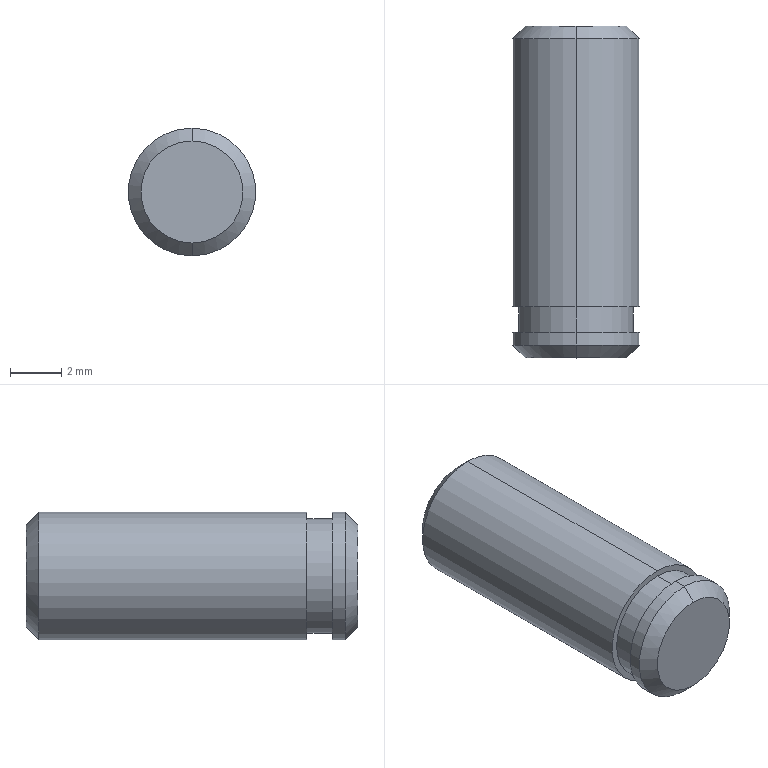Part | SolidWorks | features ICE 2, Chamfer 1, Extrusion 1 | 1 solid | 14 faces | box 5 x 13 x 5 mm | volume 247.859 mm3 | cylinder 6 | cone 4 | plane 4 | commonest cylinder face diameters 5 x4 4.5 x2
STEP:
#1=CARTESIAN_POINT('',(0.,13.,2.));
#2=VERTEX_POINT('',#1);
#3=CARTESIAN_POINT('',(0.,13.,-2.));
#4=VERTEX_POINT('',#3);
#5=CARTESIAN_POINT('',(0.,13.,0.));
#6=DIRECTION('',(0.,1.,0.));
#7=DIRECTION('',(0.,0.,1.));
#8=AXIS2_PLACEMENT_3D('',#5,#6,#7);
#9=CIRCLE('',#8,2.);
#10=EDGE_CURVE('',#2,#4,#9,.T.);
#11=ORIENTED_EDGE('',*,*,#10,.F.);
#12=CARTESIAN_POINT('',(0.,12.5,2.5));
#13=VERTEX_POINT('',#12);
#14=CARTESIAN_POINT('',(0.,13.,2.));
#15=DIRECTION('',(0.,-0.7071,0.7071));
#16=VECTOR('',#15,1000.);
#17=LINE('',#14,#16);
#18=EDGE_CURVE('',#2,#13,#17,.T.);
#19=ORIENTED_EDGE('',*,*,#18,.T.);
#20=CARTESIAN_POINT('',(0.,12.5,-2.5));
#21=VERTEX_POINT('',#20);
#22=CARTESIAN_POINT('',(0.,12.5,0.));
#23=DIRECTION('',(0.,-1.,0.));
#24=DIRECTION('',(0.,0.,1.));
#25=AXIS2_PLACEMENT_3D('',#22,#23,#24);
#26=CIRCLE('',#25,2.5);
#27=EDGE_CURVE('',#21,#13,#26,.T.);
#28=ORIENTED_EDGE('',*,*,#27,.F.);
#29=CARTESIAN_POINT('',(0.,13.,-2.));
#30=DIRECTION('',(0.,-0.7071,-0.7071));
#31=VECTOR('',#30,1000.);
#32=LINE('',#29,#31);
#33=EDGE_CURVE('',#4,#21,#32,.T.);
#34=ORIENTED_EDGE('',*,*,#33,.F.);
#35=EDGE_LOOP('',(#11,#19,#28,#34));
#36=FACE_OUTER_BOUND('',#35,.T.);
#37=CARTESIAN_POINT('',(0.,13.,0.));
#38=DIRECTION('',(0.,-1.,0.));
#39=DIRECTION('',(0.,0.,-1.));
#40=AXIS2_PLACEMENT_3D('',#37,#38,#39);
#41=CONICAL_SURFACE('',#40,2.,0.7854);
#42=ADVANCED_FACE('',(#36),#41,.T.);
#43=CARTESIAN_POINT('',(0.,0.,-2.));
#44=VERTEX_POINT('',#43);
#45=CARTESIAN_POINT('',(0.,0.,2.));
#46=VERTEX_POINT('',#45);
#47=CARTESIAN_POINT('',(0.,0.,0.));
#48=DIRECTION('',(0.,-1.,0.));
#49=DIRECTION('',(0.,0.,1.));
#50=AXIS2_PLACEMENT_3D('',#47,#48,#49);
#51=CIRCLE('',#50,2.);
#52=EDGE_CURVE('',#44,#46,#51,.T.);
#53=ORIENTED_EDGE('',*,*,#52,.F.);
#54=CARTESIAN_POINT('',(0.,0.5,-2.5));
#55=VERTEX_POINT('',#54);
#56=CARTESIAN_POINT('',(0.,0.5,-2.5));
#57=DIRECTION('',(0.,0.7071,-0.7071));
#58=VECTOR('',#57,1000.);
#59=LINE('',#56,#58);
#60=EDGE_CURVE('',#44,#55,#59,.T.);
#61=ORIENTED_EDGE('',*,*,#60,.T.);
#62=CARTESIAN_POINT('',(0.,0.5,2.5));
#63=VERTEX_POINT('',#62);
#64=CARTESIAN_POINT('',(0.,0.5,0.));
#65=DIRECTION('',(0.,1.,0.));
#66=DIRECTION('',(0.,0.,1.));
#67=AXIS2_PLACEMENT_3D('',#64,#65,#66);
#68=CIRCLE('',#67,2.5);
#69=EDGE_CURVE('',#63,#55,#68,.T.);
#70=ORIENTED_EDGE('',*,*,#69,.F.);
#71=CARTESIAN_POINT('',(0.,0.5,2.5));
#72=DIRECTION('',(0.,0.7071,0.7071));
#73=VECTOR('',#72,1000.);
#74=LINE('',#71,#73);
#75=EDGE_CURVE('',#46,#63,#74,.T.);
#76=ORIENTED_EDGE('',*,*,#75,.F.);
#77=EDGE_LOOP('',(#53,#61,#70,#76));
#78=FACE_OUTER_BOUND('',#77,.T.);
#79=CARTESIAN_POINT('',(0.,0.5,0.));
#80=DIRECTION('',(0.,1.,0.));
#81=DIRECTION('',(0.,0.,1.));
#82=AXIS2_PLACEMENT_3D('',#79,#80,#81);
#83=CONICAL_SURFACE('',#82,2.5,0.7854);
#84=ADVANCED_FACE('',(#78),#83,.T.);
#85=ORIENTED_EDGE('',*,*,#27,.T.);
#86=CARTESIAN_POINT('',(0.,2.,2.5));
#87=VERTEX_POINT('',#86);
#88=CARTESIAN_POINT('',(0.,13.,2.5));
#89=DIRECTION('',(0.,-1.,0.));
#90=VECTOR('',#89,1000.);
#91=LINE('',#88,#90);
#92=EDGE_CURVE('',#13,#87,#91,.T.);
#93=ORIENTED_EDGE('',*,*,#92,.T.);
#94=CARTESIAN_POINT('',(0.,2.,-2.5));
#95=VERTEX_POINT('',#94);
#96=CARTESIAN_POINT('',(0.,2.,0.));
#97=DIRECTION('',(0.,1.,0.));
#98=DIRECTION('',(0.,0.,1.));
#99=AXIS2_PLACEMENT_3D('',#96,#97,#98);
#100=CIRCLE('',#99,2.5);
#101=EDGE_CURVE('',#87,#95,#100,.T.);
#102=ORIENTED_EDGE('',*,*,#101,.T.);
#103=CARTESIAN_POINT('',(0.,13.,-2.5));
#104=DIRECTION('',(0.,-1.,0.));
#105=VECTOR('',#104,1000.);
#106=LINE('',#103,#105);
#107=EDGE_CURVE('',#21,#95,#106,.T.);
#108=ORIENTED_EDGE('',*,*,#107,.F.);
#109=EDGE_LOOP('',(#85,#93,#102,#108));
#110=FACE_OUTER_BOUND('',#109,.T.);
#111=CARTESIAN_POINT('',(0.,13.,0.));
#112=DIRECTION('',(0.,-1.,0.));
#113=DIRECTION('',(0.,0.,-1.));
#114=AXIS2_PLACEMENT_3D('',#111,#112,#113);
#115=CYLINDRICAL_SURFACE('',#114,2.5);
#116=ADVANCED_FACE('',(#110),#115,.T.);
#117=CARTESIAN_POINT('',(0.,2.,2.25));
#118=VERTEX_POINT('',#117);
#119=CARTESIAN_POINT('',(0.,2.,-2.25));
#120=VERTEX_POINT('',#119);
#121=CARTESIAN_POINT('',(0.,2.,0.));
#122=DIRECTION('',(0.,1.,0.));
#123=DIRECTION('',(0.,0.,1.));
#124=AXIS2_PLACEMENT_3D('',#121,#122,#123);
#125=CIRCLE('',#124,2.25);
#126=EDGE_CURVE('',#118,#120,#125,.T.);
#127=ORIENTED_EDGE('',*,*,#126,.F.);
#128=CARTESIAN_POINT('',(0.,1.,2.25));
#129=VERTEX_POINT('',#128);
#130=CARTESIAN_POINT('',(0.,2.,2.25));
#131=DIRECTION('',(0.,-1.,0.));
#132=VECTOR('',#131,1000.);
#133=LINE('',#130,#132);
#134=EDGE_CURVE('',#118,#129,#133,.T.);
#135=ORIENTED_EDGE('',*,*,#134,.T.);
#136=CARTESIAN_POINT('',(0.,1.,-2.25));
#137=VERTEX_POINT('',#136);
#138=CARTESIAN_POINT('',(0.,1.,0.));
#139=DIRECTION('',(0.,1.,0.));
#140=DIRECTION('',(0.,0.,1.));
#141=AXIS2_PLACEMENT_3D('',#138,#139,#140);
#142=CIRCLE('',#141,2.25);
#143=EDGE_CURVE('',#129,#137,#142,.T.);
#144=ORIENTED_EDGE('',*,*,#143,.T.);
#145=CARTESIAN_POINT('',(0.,2.,-2.25));
#146=DIRECTION('',(0.,-1.,0.));
#147=VECTOR('',#146,1000.);
#148=LINE('',#145,#147);
#149=EDGE_CURVE('',#120,#137,#148,.T.);
#150=ORIENTED_EDGE('',*,*,#149,.F.);
#151=EDGE_LOOP('',(#127,#135,#144,#150));
#152=FACE_OUTER_BOUND('',#151,.T.);
#153=CARTESIAN_POINT('',(0.,2.,0.));
#154=DIRECTION('',(0.,-1.,0.));
#155=DIRECTION('',(0.,0.,-1.));
#156=AXIS2_PLACEMENT_3D('',#153,#154,#155);
#157=CYLINDRICAL_SURFACE('',#156,2.25);
#158=ADVANCED_FACE('',(#152),#157,.T.);
#159=CARTESIAN_POINT('',(0.,1.,2.5));
#160=VERTEX_POINT('',#159);
#161=CARTESIAN_POINT('',(0.,1.,-2.5));
#162=VERTEX_POINT('',#161);
#163=CARTESIAN_POINT('',(0.,1.,0.));
#164=DIRECTION('',(0.,1.,0.));
#165=DIRECTION('',(0.,0.,1.));
#166=AXIS2_PLACEMENT_3D('',#163,#164,#165);
#167=CIRCLE('',#166,2.5);
#168=EDGE_CURVE('',#160,#162,#167,.T.);
#169=ORIENTED_EDGE('',*,*,#168,.F.);
#170=CARTESIAN_POINT('',(0.,1.,2.5));
#171=DIRECTION('',(0.,-1.,0.));
#172=VECTOR('',#171,1000.);
#173=LINE('',#170,#172);
#174=EDGE_CURVE('',#160,#63,#173,.T.);
#175=ORIENTED_EDGE('',*,*,#174,.T.);
#176=ORIENTED_EDGE('',*,*,#69,.T.);
#177=CARTESIAN_POINT('',(0.,1.,-2.5));
#178=DIRECTION('',(0.,-1.,0.));
#179=VECTOR('',#178,1000.);
#180=LINE('',#177,#179);
#181=EDGE_CURVE('',#162,#55,#180,.T.);
#182=ORIENTED_EDGE('',*,*,#181,.F.);
#183=EDGE_LOOP('',(#169,#175,#176,#182));
#184=FACE_OUTER_BOUND('',#183,.T.);
#185=CARTESIAN_POINT('',(0.,1.,0.));
#186=DIRECTION('',(0.,-1.,0.));
#187=DIRECTION('',(0.,0.,-1.));
#188=AXIS2_PLACEMENT_3D('',#185,#186,#187);
#189=CYLINDRICAL_SURFACE('',#188,2.5);
#190=ADVANCED_FACE('',(#184),#189,.T.);
#191=ORIENTED_EDGE('',*,*,#174,.F.);
#192=CARTESIAN_POINT('',(0.,1.,0.));
#193=DIRECTION('',(0.,1.,0.));
#194=DIRECTION('',(0.,0.,1.));
#195=AXIS2_PLACEMENT_3D('',#192,#193,#194);
#196=CIRCLE('',#195,2.5);
#197=EDGE_CURVE('',#162,#160,#196,.T.);
#198=ORIENTED_EDGE('',*,*,#197,.F.);
#199=ORIENTED_EDGE('',*,*,#181,.T.);
#200=CARTESIAN_POINT('',(0.,0.5,0.));
#201=DIRECTION('',(0.,1.,0.));
#202=DIRECTION('',(0.,0.,1.));
#203=AXIS2_PLACEMENT_3D('',#200,#201,#202);
#204=CIRCLE('',#203,2.5);
#205=EDGE_CURVE('',#55,#63,#204,.T.);
#206=ORIENTED_EDGE('',*,*,#205,.T.);
#207=EDGE_LOOP('',(#191,#198,#199,#206));
#208=FACE_OUTER_BOUND('',#207,.T.);
#209=CARTESIAN_POINT('',(0.,1.,0.));
#210=DIRECTION('',(0.,-1.,0.));
#211=DIRECTION('',(0.,0.,-1.));
#212=AXIS2_PLACEMENT_3D('',#209,#210,#211);
#213=CYLINDRICAL_SURFACE('',#212,2.5);
#214=ADVANCED_FACE('',(#208),#213,.T.);
#215=CARTESIAN_POINT('',(0.,1.,0.));
#216=DIRECTION('',(0.,1.,0.));
#217=DIRECTION('',(0.,0.,1.));
#218=AXIS2_PLACEMENT_3D('',#215,#216,#217);
#219=CIRCLE('',#218,2.25);
#220=EDGE_CURVE('',#137,#129,#219,.T.);
#221=ORIENTED_EDGE('',*,*,#220,.F.);
#222=ORIENTED_EDGE('',*,*,#143,.F.);
#223=EDGE_LOOP('',(#221,#222));
#224=FACE_BOUND('',#223,.T.);
#225=ORIENTED_EDGE('',*,*,#197,.T.);
#226=ORIENTED_EDGE('',*,*,#168,.T.);
#227=EDGE_LOOP('',(#225,#226));
#228=FACE_OUTER_BOUND('',#227,.T.);
#229=CARTESIAN_POINT('',(0.,1.,0.));
#230=DIRECTION('',(0.,1.,0.));
#231=DIRECTION('',(0.,0.,1.));
#232=AXIS2_PLACEMENT_3D('',#229,#230,#231);
#233=PLANE('',#232);
#234=ADVANCED_FACE('',(#224,#228),#233,.T.);
#235=CARTESIAN_POINT('',(0.,0.,0.));
#236=DIRECTION('',(0.,-1.,0.));
#237=DIRECTION('',(0.,0.,1.));
#238=AXIS2_PLACEMENT_3D('',#235,#236,#237);
#239=CIRCLE('',#238,2.);
#240=EDGE_CURVE('',#46,#44,#239,.T.);
#241=ORIENTED_EDGE('',*,*,#240,.T.);
#242=ORIENTED_EDGE('',*,*,#52,.T.);
#243=EDGE_LOOP('',(#241,#242));
#244=FACE_OUTER_BOUND('',#243,.T.);
#245=CARTESIAN_POINT('',(0.,0.,0.));
#246=DIRECTION('',(0.,1.,0.));
#247=DIRECTION('',(0.,0.,1.));
#248=AXIS2_PLACEMENT_3D('',#245,#246,#247);
#249=PLANE('',#248);
#250=ADVANCED_FACE('',(#244),#249,.F.);
#251=ORIENTED_EDGE('',*,*,#134,.F.);
#252=CARTESIAN_POINT('',(0.,2.,0.));
#253=DIRECTION('',(0.,1.,0.));
#254=DIRECTION('',(0.,0.,1.));
#255=AXIS2_PLACEMENT_3D('',#252,#253,#254);
#256=CIRCLE('',#255,2.25);
#257=EDGE_CURVE('',#120,#118,#256,.T.);
#258=ORIENTED_EDGE('',*,*,#257,.F.);
#259=ORIENTED_EDGE('',*,*,#149,.T.);
#260=ORIENTED_EDGE('',*,*,#220,.T.);
#261=EDGE_LOOP('',(#251,#258,#259,#260));
#262=FACE_OUTER_BOUND('',#261,.T.);
#263=CARTESIAN_POINT('',(0.,2.,0.));
#264=DIRECTION('',(0.,-1.,0.));
#265=DIRECTION('',(0.,0.,-1.));
#266=AXIS2_PLACEMENT_3D('',#263,#264,#265);
#267=CYLINDRICAL_SURFACE('',#266,2.25);
#268=ADVANCED_FACE('',(#262),#267,.T.);
#269=ORIENTED_EDGE('',*,*,#92,.F.);
#270=CARTESIAN_POINT('',(0.,12.5,0.));
#271=DIRECTION('',(0.,-1.,0.));
#272=DIRECTION('',(0.,0.,1.));
#273=AXIS2_PLACEMENT_3D('',#270,#271,#272);
#274=CIRCLE('',#273,2.5);
#275=EDGE_CURVE('',#13,#21,#274,.T.);
#276=ORIENTED_EDGE('',*,*,#275,.T.);
#277=ORIENTED_EDGE('',*,*,#107,.T.);
#278=CARTESIAN_POINT('',(0.,2.,0.));
#279=DIRECTION('',(0.,1.,0.));
#280=DIRECTION('',(0.,0.,1.));
#281=AXIS2_PLACEMENT_3D('',#278,#279,#280);
#282=CIRCLE('',#281,2.5);
#283=EDGE_CURVE('',#95,#87,#282,.T.);
#284=ORIENTED_EDGE('',*,*,#283,.T.);
#285=EDGE_LOOP('',(#269,#276,#277,#284));
#286=FACE_OUTER_BOUND('',#285,.T.);
#287=CARTESIAN_POINT('',(0.,13.,0.));
#288=DIRECTION('',(0.,-1.,0.));
#289=DIRECTION('',(0.,0.,-1.));
#290=AXIS2_PLACEMENT_3D('',#287,#288,#289);
#291=CYLINDRICAL_SURFACE('',#290,2.5);
#292=ADVANCED_FACE('',(#286),#291,.T.);
#293=CARTESIAN_POINT('',(0.,13.,0.));
#294=DIRECTION('',(0.,1.,0.));
#295=DIRECTION('',(0.,0.,1.));
#296=AXIS2_PLACEMENT_3D('',#293,#294,#295);
#297=CIRCLE('',#296,2.);
#298=EDGE_CURVE('',#4,#2,#297,.T.);
#299=ORIENTED_EDGE('',*,*,#298,.T.);
#300=ORIENTED_EDGE('',*,*,#10,.T.);
#301=EDGE_LOOP('',(#299,#300));
#302=FACE_OUTER_BOUND('',#301,.T.);
#303=CARTESIAN_POINT('',(0.,13.,0.));
#304=DIRECTION('',(0.,1.,0.));
#305=DIRECTION('',(0.,0.,1.));
#306=AXIS2_PLACEMENT_3D('',#303,#304,#305);
#307=PLANE('',#306);
#308=ADVANCED_FACE('',(#302),#307,.T.);
#309=ORIENTED_EDGE('',*,*,#257,.T.);
#310=ORIENTED_EDGE('',*,*,#126,.T.);
#311=EDGE_LOOP('',(#309,#310));
#312=FACE_BOUND('',#311,.T.);
#313=ORIENTED_EDGE('',*,*,#283,.F.);
#314=ORIENTED_EDGE('',*,*,#101,.F.);
#315=EDGE_LOOP('',(#313,#314));
#316=FACE_OUTER_BOUND('',#315,.T.);
#317=CARTESIAN_POINT('',(0.,2.,0.));
#318=DIRECTION('',(0.,1.,0.));
#319=DIRECTION('',(0.,0.,1.));
#320=AXIS2_PLACEMENT_3D('',#317,#318,#319);
#321=PLANE('',#320);
#322=ADVANCED_FACE('',(#312,#316),#321,.F.);
#323=ORIENTED_EDGE('',*,*,#60,.F.);
#324=ORIENTED_EDGE('',*,*,#240,.F.);
#325=ORIENTED_EDGE('',*,*,#75,.T.);
#326=ORIENTED_EDGE('',*,*,#205,.F.);
#327=EDGE_LOOP('',(#323,#324,#325,#326));
#328=FACE_OUTER_BOUND('',#327,.T.);
#329=CARTESIAN_POINT('',(0.,0.5,0.));
#330=DIRECTION('',(0.,1.,0.));
#331=DIRECTION('',(0.,0.,1.));
#332=AXIS2_PLACEMENT_3D('',#329,#330,#331);
#333=CONICAL_SURFACE('',#332,2.5,0.7854);
#334=ADVANCED_FACE('',(#328),#333,.T.);
#335=ORIENTED_EDGE('',*,*,#18,.F.);
#336=ORIENTED_EDGE('',*,*,#298,.F.);
#337=ORIENTED_EDGE('',*,*,#33,.T.);
#338=ORIENTED_EDGE('',*,*,#275,.F.);
#339=EDGE_LOOP('',(#335,#336,#337,#338));
#340=FACE_OUTER_BOUND('',#339,.T.);
#341=CARTESIAN_POINT('',(0.,13.,0.));
#342=DIRECTION('',(0.,-1.,0.));
#343=DIRECTION('',(0.,0.,-1.));
#344=AXIS2_PLACEMENT_3D('',#341,#342,#343);
#345=CONICAL_SURFACE('',#344,2.,0.7854);
#346=ADVANCED_FACE('',(#340),#345,.T.);
#347=CLOSED_SHELL('',(#42,#84,#116,#158,#190,#214,#234,#250,#268,#292,#308,#322,#334,#346));
#348=MANIFOLD_SOLID_BREP('',#347);
#349=CARTESIAN_POINT('',(0.,0.,0.));
#350=DIRECTION('',(0.,0.,1.));
#351=DIRECTION('',(1.,0.,0.));
#352=AXIS2_PLACEMENT_3D('',#349,#350,#351);
#353=(LENGTH_UNIT()NAMED_UNIT(*)SI_UNIT(.MILLI.,.METRE.));
#354=UNCERTAINTY_MEASURE_WITH_UNIT(LENGTH_MEASURE(0.00001),#353,'','');
#355=(NAMED_UNIT(*)PLANE_ANGLE_UNIT()SI_UNIT($,.RADIAN.));
#356=(NAMED_UNIT(*)SI_UNIT($,.STERADIAN.)SOLID_ANGLE_UNIT());
#357=(GEOMETRIC_REPRESENTATION_CONTEXT(3)GLOBAL_UNCERTAINTY_ASSIGNED_CONTEXT((#354))GLOBAL_UNIT_ASSIGNED_CONTEXT((#353,#355,#356))REPRESENTATION_CONTEXT('',''));
#358=ADVANCED_BREP_SHAPE_REPRESENTATION('',(#348,#352),#357);